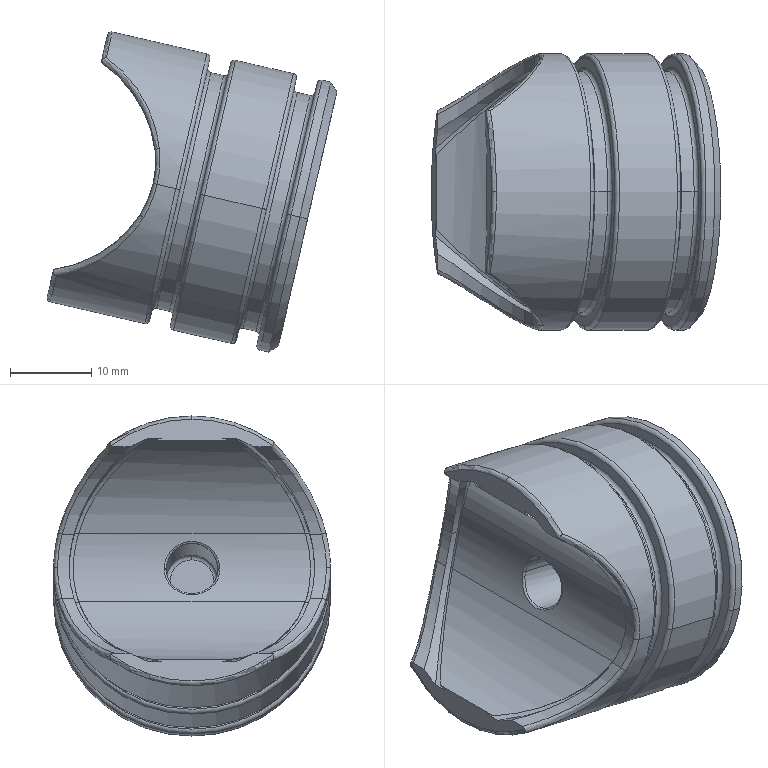Part | SolidWorks | features BaseBody 1 | 1 solid | 91 faces | box 35.548 x 33.98 x 39.287 mm | volume 16613 mm3 | cylinder 37 | torus 32 | plane 10 | spline 10 | cone 2 | commonest cylinder face diameters 33.98 x6 29.7 x4 31.883 x4 29.12 x3 30.12 x3 6.35 x2